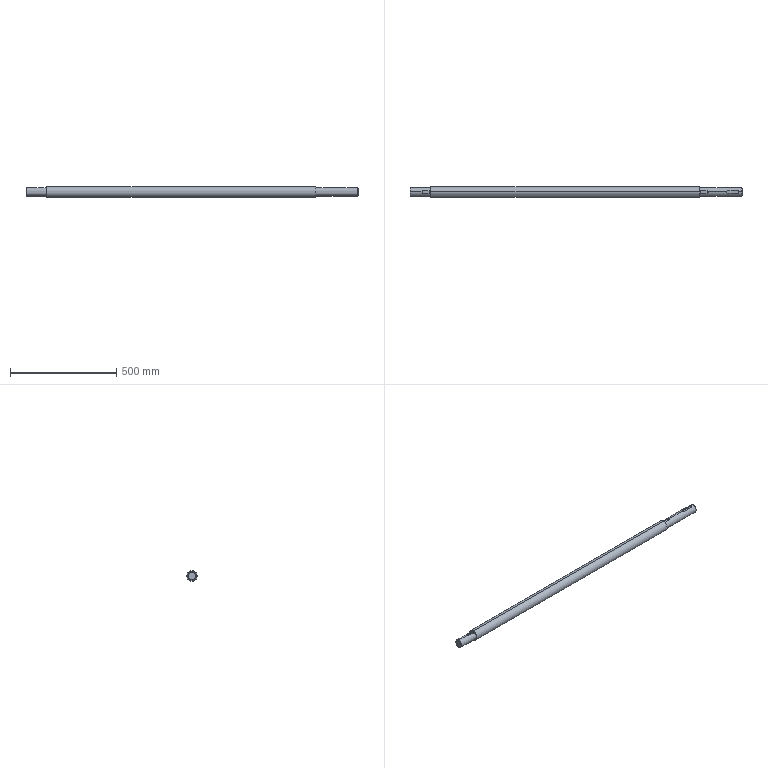Part | STEP file | Produce dryer mesh belt driving shaft | 1 solid | 32 faces | box 1562 x 50 x 50 mm | volume 2850228 mm3 | cylinder 15 | plane 13 | cone 4 | commonest cylinder face diameters 12 x9 40 x4 50 x2
STEP:
#1=CARTESIAN_POINT('',(832.25,0.,-18.));
#2=VERTEX_POINT('',#1);
#3=CARTESIAN_POINT('',(832.25,0.,18.));
#4=VERTEX_POINT('',#3);
#5=CARTESIAN_POINT('',(832.25,0.,0.));
#6=DIRECTION('',(1.,0.,0.));
#7=DIRECTION('',(0.,0.,1.));
#8=AXIS2_PLACEMENT_3D('',#5,#6,#7);
#9=CIRCLE('',#8,18.);
#10=EDGE_CURVE('',#2,#4,#9,.T.);
#11=ORIENTED_EDGE('',*,*,#10,.F.);
#12=CARTESIAN_POINT('',(830.25,0.,-20.));
#13=VERTEX_POINT('',#12);
#14=CARTESIAN_POINT('',(830.25,0.,-20.));
#15=DIRECTION('',(-0.7071,0.,-0.7071));
#16=VECTOR('',#15,1000.);
#17=LINE('',#14,#16);
#18=EDGE_CURVE('',#2,#13,#17,.T.);
#19=ORIENTED_EDGE('',*,*,#18,.T.);
#20=CARTESIAN_POINT('',(830.25,0.,20.));
#21=VERTEX_POINT('',#20);
#22=CARTESIAN_POINT('',(830.25,0.,0.));
#23=DIRECTION('',(-1.,0.,0.));
#24=DIRECTION('',(0.,0.,1.));
#25=AXIS2_PLACEMENT_3D('',#22,#23,#24);
#26=CIRCLE('',#25,20.);
#27=EDGE_CURVE('',#21,#13,#26,.T.);
#28=ORIENTED_EDGE('',*,*,#27,.F.);
#29=CARTESIAN_POINT('',(830.25,0.,20.));
#30=DIRECTION('',(-0.7071,0.,0.7071));
#31=VECTOR('',#30,1000.);
#32=LINE('',#29,#31);
#33=EDGE_CURVE('',#4,#21,#32,.T.);
#34=ORIENTED_EDGE('',*,*,#33,.F.);
#35=EDGE_LOOP('',(#11,#19,#28,#34));
#36=FACE_OUTER_BOUND('',#35,.T.);
#37=CARTESIAN_POINT('',(830.25,0.,0.));
#38=DIRECTION('',(-1.,0.,0.));
#39=DIRECTION('',(0.,0.,1.));
#40=AXIS2_PLACEMENT_3D('',#37,#38,#39);
#41=CONICAL_SURFACE('',#40,20.,0.7854);
#42=ADVANCED_FACE('',(#36),#41,.T.);
#43=CARTESIAN_POINT('',(-730.25,0.,18.));
#44=VERTEX_POINT('',#43);
#45=CARTESIAN_POINT('',(-730.25,0.,-18.));
#46=VERTEX_POINT('',#45);
#47=CARTESIAN_POINT('',(-730.25,0.,0.));
#48=DIRECTION('',(-1.,0.,0.));
#49=DIRECTION('',(0.,0.,-1.));
#50=AXIS2_PLACEMENT_3D('',#47,#48,#49);
#51=CIRCLE('',#50,18.);
#52=EDGE_CURVE('',#44,#46,#51,.T.);
#53=ORIENTED_EDGE('',*,*,#52,.F.);
#54=CARTESIAN_POINT('',(-728.25,0.,20.));
#55=VERTEX_POINT('',#54);
#56=CARTESIAN_POINT('',(-730.25,0.,18.));
#57=DIRECTION('',(0.7071,0.,0.7071));
#58=VECTOR('',#57,1000.);
#59=LINE('',#56,#58);
#60=EDGE_CURVE('',#44,#55,#59,.T.);
#61=ORIENTED_EDGE('',*,*,#60,.T.);
#62=CARTESIAN_POINT('',(-728.25,0.,-20.));
#63=VERTEX_POINT('',#62);
#64=CARTESIAN_POINT('',(-728.25,0.,0.));
#65=DIRECTION('',(1.,0.,0.));
#66=DIRECTION('',(0.,0.,-1.));
#67=AXIS2_PLACEMENT_3D('',#64,#65,#66);
#68=CIRCLE('',#67,20.);
#69=EDGE_CURVE('',#63,#55,#68,.T.);
#70=ORIENTED_EDGE('',*,*,#69,.F.);
#71=CARTESIAN_POINT('',(-730.25,0.,-18.));
#72=DIRECTION('',(0.7071,0.,-0.7071));
#73=VECTOR('',#72,1000.);
#74=LINE('',#71,#73);
#75=EDGE_CURVE('',#46,#63,#74,.T.);
#76=ORIENTED_EDGE('',*,*,#75,.F.);
#77=EDGE_LOOP('',(#53,#61,#70,#76));
#78=FACE_OUTER_BOUND('',#77,.T.);
#79=CARTESIAN_POINT('',(-730.25,0.,0.));
#80=DIRECTION('',(1.,0.,0.));
#81=DIRECTION('',(0.,0.,-1.));
#82=AXIS2_PLACEMENT_3D('',#79,#80,#81);
#83=CONICAL_SURFACE('',#82,18.,0.7854);
#84=ADVANCED_FACE('',(#78),#83,.T.);
#85=CARTESIAN_POINT('',(673.75,0.,15.));
#86=VERTEX_POINT('',#85);
#87=CARTESIAN_POINT('',(667.75,6.,15.));
#88=VERTEX_POINT('',#87);
#89=CARTESIAN_POINT('',(667.75,0.,15.));
#90=DIRECTION('',(0.,0.,1.));
#91=DIRECTION('',(-1.,0.,0.));
#92=AXIS2_PLACEMENT_3D('',#89,#90,#91);
#93=CIRCLE('',#92,6.);
#94=EDGE_CURVE('',#86,#88,#93,.T.);
#95=ORIENTED_EDGE('',*,*,#94,.F.);
#96=CARTESIAN_POINT('',(673.75,0.,20.));
#97=VERTEX_POINT('',#96);
#98=CARTESIAN_POINT('',(673.75,0.,15.));
#99=DIRECTION('',(0.,0.,1.));
#100=VECTOR('',#99,1000.);
#101=LINE('',#98,#100);
#102=EDGE_CURVE('',#86,#97,#101,.T.);
#103=ORIENTED_EDGE('',*,*,#102,.T.);
#104=CARTESIAN_POINT('',(667.75,6.,19.079));
#105=VERTEX_POINT('',#104);
#106=CARTESIAN_POINT('',(667.75,6.,19.079));
#107=CARTESIAN_POINT('',(668.145,6.,19.079));
#108=CARTESIAN_POINT('',(668.536,5.961,19.091));
#109=CARTESIAN_POINT('',(669.116,5.846,19.127));
#110=CARTESIAN_POINT('',(669.309,5.797,19.141));
#111=CARTESIAN_POINT('',(669.688,5.682,19.176));
#112=CARTESIAN_POINT('',(669.873,5.615,19.196));
#113=CARTESIAN_POINT('',(670.415,5.39,19.261));
#114=CARTESIAN_POINT('',(670.759,5.206,19.312));
#115=CARTESIAN_POINT('',(671.415,4.767,19.425));
#116=CARTESIAN_POINT('',(671.716,4.519,19.485));
#117=CARTESIAN_POINT('',(672.129,4.107,19.574));
#118=CARTESIAN_POINT('',(672.26,3.962,19.604));
#119=CARTESIAN_POINT('',(672.509,3.66,19.663));
#120=CARTESIAN_POINT('',(672.627,3.501,19.692));
#121=CARTESIAN_POINT('',(672.953,3.013,19.775));
#122=CARTESIAN_POINT('',(673.138,2.67,19.824));
#123=CARTESIAN_POINT('',(673.439,1.946,19.908));
#124=CARTESIAN_POINT('',(673.556,1.563,19.943));
#125=CARTESIAN_POINT('',(673.711,0.7911,19.988));
#126=CARTESIAN_POINT('',(673.75,0.3988,20.));
#127=CARTESIAN_POINT('',(673.75,0.,20.));
#128=B_SPLINE_CURVE_WITH_KNOTS('',3,(#106,#107,#108,#109,#110,#111,#112,#113,#114,#115,#116,#117,#118,#119,#120,#121,#122,#123,#124,#125,#126,#127),.UNSPECIFIED.,.F.,.F.,(4,2,2,2,2,2,2,2,2,2,4),(0.0283,0.02948,0.03007,0.03066,0.03184,0.03302,0.0336,0.03419,0.03537,0.03655,0.03773),.UNSPECIFIED.);
#129=EDGE_CURVE('',#105,#97,#128,.T.);
#130=ORIENTED_EDGE('',*,*,#129,.F.);
#131=CARTESIAN_POINT('',(667.75,6.,15.));
#132=DIRECTION('',(0.,0.,1.));
#133=VECTOR('',#132,1000.);
#134=LINE('',#131,#133);
#135=EDGE_CURVE('',#88,#105,#134,.T.);
#136=ORIENTED_EDGE('',*,*,#135,.F.);
#137=EDGE_LOOP('',(#95,#103,#130,#136));
#138=FACE_OUTER_BOUND('',#137,.T.);
#139=CARTESIAN_POINT('',(667.75,0.,15.));
#140=DIRECTION('',(0.,0.,1.));
#141=DIRECTION('',(1.,0.,0.));
#142=AXIS2_PLACEMENT_3D('',#139,#140,#141);
#143=CYLINDRICAL_SURFACE('',#142,6.);
#144=ADVANCED_FACE('',(#138),#143,.F.);
#145=CARTESIAN_POINT('',(818.25,0.,15.));
#146=VERTEX_POINT('',#145);
#147=CARTESIAN_POINT('',(812.25,6.,15.));
#148=VERTEX_POINT('',#147);
#149=CARTESIAN_POINT('',(812.25,0.,15.));
#150=DIRECTION('',(0.,0.,1.));
#151=DIRECTION('',(1.,0.,0.));
#152=AXIS2_PLACEMENT_3D('',#149,#150,#151);
#153=CIRCLE('',#152,6.);
#154=EDGE_CURVE('',#146,#148,#153,.T.);
#155=ORIENTED_EDGE('',*,*,#154,.F.);
#156=CARTESIAN_POINT('',(818.25,0.,20.));
#157=VERTEX_POINT('',#156);
#158=CARTESIAN_POINT('',(818.25,0.,15.));
#159=DIRECTION('',(0.,0.,1.));
#160=VECTOR('',#159,1000.);
#161=LINE('',#158,#160);
#162=EDGE_CURVE('',#146,#157,#161,.T.);
#163=ORIENTED_EDGE('',*,*,#162,.T.);
#164=CARTESIAN_POINT('',(812.25,6.,19.079));
#165=VERTEX_POINT('',#164);
#166=CARTESIAN_POINT('',(812.25,6.,19.079));
#167=CARTESIAN_POINT('',(812.645,6.,19.079));
#168=CARTESIAN_POINT('',(813.036,5.961,19.091));
#169=CARTESIAN_POINT('',(813.616,5.846,19.127));
#170=CARTESIAN_POINT('',(813.809,5.797,19.141));
#171=CARTESIAN_POINT('',(814.188,5.682,19.176));
#172=CARTESIAN_POINT('',(814.373,5.615,19.196));
#173=CARTESIAN_POINT('',(814.915,5.39,19.261));
#174=CARTESIAN_POINT('',(815.259,5.206,19.312));
#175=CARTESIAN_POINT('',(815.915,4.767,19.425));
#176=CARTESIAN_POINT('',(816.216,4.519,19.485));
#177=CARTESIAN_POINT('',(816.629,4.107,19.574));
#178=CARTESIAN_POINT('',(816.76,3.962,19.604));
#179=CARTESIAN_POINT('',(817.009,3.66,19.663));
#180=CARTESIAN_POINT('',(817.127,3.501,19.692));
#181=CARTESIAN_POINT('',(817.453,3.013,19.775));
#182=CARTESIAN_POINT('',(817.638,2.67,19.824));
#183=CARTESIAN_POINT('',(817.939,1.946,19.908));
#184=CARTESIAN_POINT('',(818.056,1.563,19.943));
#185=CARTESIAN_POINT('',(818.211,0.7911,19.988));
#186=CARTESIAN_POINT('',(818.25,0.3988,20.));
#187=CARTESIAN_POINT('',(818.25,0.,20.));
#188=B_SPLINE_CURVE_WITH_KNOTS('',3,(#166,#167,#168,#169,#170,#171,#172,#173,#174,#175,#176,#177,#178,#179,#180,#181,#182,#183,#184,#185,#186,#187),.UNSPECIFIED.,.F.,.F.,(4,2,2,2,2,2,2,2,2,2,4),(0.0283,0.02948,0.03007,0.03066,0.03184,0.03302,0.0336,0.03419,0.03537,0.03655,0.03773),.UNSPECIFIED.);
#189=EDGE_CURVE('',#165,#157,#188,.T.);
#190=ORIENTED_EDGE('',*,*,#189,.F.);
#191=CARTESIAN_POINT('',(812.25,6.,15.));
#192=DIRECTION('',(0.,0.,1.));
#193=VECTOR('',#192,1000.);
#194=LINE('',#191,#193);
#195=EDGE_CURVE('',#148,#165,#194,.T.);
#196=ORIENTED_EDGE('',*,*,#195,.F.);
#197=EDGE_LOOP('',(#155,#163,#190,#196));
#198=FACE_OUTER_BOUND('',#197,.T.);
#199=CARTESIAN_POINT('',(812.25,0.,15.));
#200=DIRECTION('',(0.,0.,1.));
#201=DIRECTION('',(1.,0.,0.));
#202=AXIS2_PLACEMENT_3D('',#199,#200,#201);
#203=CYLINDRICAL_SURFACE('',#202,6.);
#204=ADVANCED_FACE('',(#198),#203,.F.);
#205=CARTESIAN_POINT('',(-634.75,0.,15.));
#206=VERTEX_POINT('',#205);
#207=CARTESIAN_POINT('',(-640.75,6.,15.));
#208=VERTEX_POINT('',#207);
#209=CARTESIAN_POINT('',(-640.75,0.,15.));
#210=DIRECTION('',(0.,0.,1.));
#211=DIRECTION('',(1.,0.,0.));
#212=AXIS2_PLACEMENT_3D('',#209,#210,#211);
#213=CIRCLE('',#212,6.);
#214=EDGE_CURVE('',#206,#208,#213,.T.);
#215=ORIENTED_EDGE('',*,*,#214,.F.);
#216=CARTESIAN_POINT('',(-634.75,0.,20.));
#217=VERTEX_POINT('',#216);
#218=CARTESIAN_POINT('',(-634.75,0.,15.));
#219=DIRECTION('',(0.,0.,1.));
#220=VECTOR('',#219,1000.);
#221=LINE('',#218,#220);
#222=EDGE_CURVE('',#206,#217,#221,.T.);
#223=ORIENTED_EDGE('',*,*,#222,.T.);
#224=CARTESIAN_POINT('',(-640.75,6.,19.079));
#225=VERTEX_POINT('',#224);
#226=CARTESIAN_POINT('',(-640.75,6.,19.079));
#227=CARTESIAN_POINT('',(-640.355,6.,19.079));
#228=CARTESIAN_POINT('',(-639.964,5.961,19.091));
#229=CARTESIAN_POINT('',(-639.384,5.846,19.127));
#230=CARTESIAN_POINT('',(-639.191,5.797,19.141));
#231=CARTESIAN_POINT('',(-638.812,5.682,19.176));
#232=CARTESIAN_POINT('',(-638.627,5.615,19.196));
#233=CARTESIAN_POINT('',(-638.085,5.39,19.261));
#234=CARTESIAN_POINT('',(-637.741,5.206,19.312));
#235=CARTESIAN_POINT('',(-637.085,4.767,19.425));
#236=CARTESIAN_POINT('',(-636.784,4.519,19.485));
#237=CARTESIAN_POINT('',(-636.371,4.107,19.574));
#238=CARTESIAN_POINT('',(-636.24,3.962,19.604));
#239=CARTESIAN_POINT('',(-635.991,3.66,19.663));
#240=CARTESIAN_POINT('',(-635.873,3.501,19.692));
#241=CARTESIAN_POINT('',(-635.547,3.013,19.775));
#242=CARTESIAN_POINT('',(-635.362,2.67,19.824));
#243=CARTESIAN_POINT('',(-635.061,1.946,19.908));
#244=CARTESIAN_POINT('',(-634.944,1.563,19.943));
#245=CARTESIAN_POINT('',(-634.789,0.7911,19.988));
#246=CARTESIAN_POINT('',(-634.75,0.3988,20.));
#247=CARTESIAN_POINT('',(-634.75,0.,20.));
#248=B_SPLINE_CURVE_WITH_KNOTS('',3,(#226,#227,#228,#229,#230,#231,#232,#233,#234,#235,#236,#237,#238,#239,#240,#241,#242,#243,#244,#245,#246,#247),.UNSPECIFIED.,.F.,.F.,(4,2,2,2,2,2,2,2,2,2,4),(0.0283,0.02948,0.03007,0.03066,0.03184,0.03302,0.0336,0.03419,0.03537,0.03655,0.03773),.UNSPECIFIED.);
#249=EDGE_CURVE('',#225,#217,#248,.T.);
#250=ORIENTED_EDGE('',*,*,#249,.F.);
#251=CARTESIAN_POINT('',(-640.75,6.,15.));
#252=DIRECTION('',(0.,0.,1.));
#253=VECTOR('',#252,1000.);
#254=LINE('',#251,#253);
#255=EDGE_CURVE('',#208,#225,#254,.T.);
#256=ORIENTED_EDGE('',*,*,#255,.F.);
#257=EDGE_LOOP('',(#215,#223,#250,#256));
#258=FACE_OUTER_BOUND('',#257,.T.);
#259=CARTESIAN_POINT('',(-640.75,0.,15.));
#260=DIRECTION('',(0.,0.,1.));
#261=DIRECTION('',(1.,0.,0.));
#262=AXIS2_PLACEMENT_3D('',#259,#260,#261);
#263=CYLINDRICAL_SURFACE('',#262,6.);
#264=ADVANCED_FACE('',(#258),#263,.F.);
#265=CARTESIAN_POINT('',(-632.75,0.,20.));
#266=VERTEX_POINT('',#265);
#267=CARTESIAN_POINT('',(-632.75,0.,-20.));
#268=VERTEX_POINT('',#267);
#269=CARTESIAN_POINT('',(-632.75,0.,0.));
#270=DIRECTION('',(-1.,0.,0.));
#271=DIRECTION('',(0.,0.,1.));
#272=AXIS2_PLACEMENT_3D('',#269,#270,#271);
#273=CIRCLE('',#272,20.);
#274=EDGE_CURVE('',#266,#268,#273,.T.);
#275=ORIENTED_EDGE('',*,*,#274,.T.);
#276=CARTESIAN_POINT('',(-832.25,0.,-20.));
#277=DIRECTION('',(-1.,0.,0.));
#278=VECTOR('',#277,1000.);
#279=LINE('',#276,#278);
#280=EDGE_CURVE('',#268,#63,#279,.T.);
#281=ORIENTED_EDGE('',*,*,#280,.T.);
#282=ORIENTED_EDGE('',*,*,#69,.T.);
#283=CARTESIAN_POINT('',(-673.75,0.,20.));
#284=VERTEX_POINT('',#283);
#285=CARTESIAN_POINT('',(-832.25,0.,20.));
#286=DIRECTION('',(-1.,0.,0.));
#287=VECTOR('',#286,1000.);
#288=LINE('',#285,#287);
#289=EDGE_CURVE('',#284,#55,#288,.T.);
#290=ORIENTED_EDGE('',*,*,#289,.F.);
#291=CARTESIAN_POINT('',(-667.75,6.,19.079));
#292=VERTEX_POINT('',#291);
#293=CARTESIAN_POINT('',(-673.75,0.,20.));
#294=CARTESIAN_POINT('',(-673.75,0.3936,20.));
#295=CARTESIAN_POINT('',(-673.71,0.7934,19.988));
#296=CARTESIAN_POINT('',(-673.556,1.564,19.942));
#297=CARTESIAN_POINT('',(-673.442,1.939,19.909));
#298=CARTESIAN_POINT('',(-673.139,2.668,19.825));
#299=CARTESIAN_POINT('',(-672.952,3.015,19.774));
#300=CARTESIAN_POINT('',(-672.627,3.5,19.692));
#301=CARTESIAN_POINT('',(-672.511,3.657,19.664));
#302=CARTESIAN_POINT('',(-672.263,3.959,19.605));
#303=CARTESIAN_POINT('',(-672.13,4.105,19.575));
#304=CARTESIAN_POINT('',(-671.715,4.52,19.485));
#305=CARTESIAN_POINT('',(-671.415,4.766,19.425));
#306=CARTESIAN_POINT('',(-670.768,5.201,19.313));
#307=CARTESIAN_POINT('',(-670.417,5.389,19.261));
#308=CARTESIAN_POINT('',(-669.695,5.69,19.174));
#309=CARTESIAN_POINT('',(-669.321,5.804,19.139));
#310=CARTESIAN_POINT('',(-668.547,5.96,19.092));
#311=CARTESIAN_POINT('',(-668.149,6.,19.079));
#312=CARTESIAN_POINT('',(-667.75,6.,19.079));
#313=B_SPLINE_CURVE_WITH_KNOTS('',3,(#293,#294,#295,#296,#297,#298,#299,#300,#301,#302,#303,#304,#305,#306,#307,#308,#309,#310,#311,#312),.UNSPECIFIED.,.F.,.F.,(4,2,2,2,2,2,2,2,2,4),(0.009436,0.01061,0.01179,0.01297,0.01356,0.01415,0.01533,0.0165,0.01768,0.01886),.UNSPECIFIED.);
#314=EDGE_CURVE('',#284,#292,#313,.T.);
#315=ORIENTED_EDGE('',*,*,#314,.T.);
#316=CARTESIAN_POINT('',(-832.25,6.,19.079));
#317=DIRECTION('',(1.,0.,0.));
#318=VECTOR('',#317,1000.);
#319=LINE('',#316,#318);
#320=EDGE_CURVE('',#292,#225,#319,.T.);
#321=ORIENTED_EDGE('',*,*,#320,.T.);
#322=ORIENTED_EDGE('',*,*,#249,.T.);
#323=CARTESIAN_POINT('',(-832.25,0.,20.));
#324=DIRECTION('',(-1.,0.,0.));
#325=VECTOR('',#324,1000.);
#326=LINE('',#323,#325);
#327=EDGE_CURVE('',#266,#217,#326,.T.);
#328=ORIENTED_EDGE('',*,*,#327,.F.);
#329=EDGE_LOOP('',(#275,#281,#282,#290,#315,#321,#322,#328));
#330=FACE_OUTER_BOUND('',#329,.T.);
#331=CARTESIAN_POINT('',(-832.25,0.,0.));
#332=DIRECTION('',(-1.,0.,0.));
#333=DIRECTION('',(0.,0.,1.));
#334=AXIS2_PLACEMENT_3D('',#331,#332,#333);
#335=CYLINDRICAL_SURFACE('',#334,20.);
#336=ADVANCED_FACE('',(#330),#335,.T.);
#337=CARTESIAN_POINT('',(632.75,0.,25.));
#338=VERTEX_POINT('',#337);
#339=CARTESIAN_POINT('',(632.75,0.,-25.));
#340=VERTEX_POINT('',#339);
#341=CARTESIAN_POINT('',(632.75,0.,0.));
#342=DIRECTION('',(-1.,0.,0.));
#343=DIRECTION('',(0.,0.,1.));
#344=AXIS2_PLACEMENT_3D('',#341,#342,#343);
#345=CIRCLE('',#344,25.);
#346=EDGE_CURVE('',#338,#340,#345,.T.);
#347=ORIENTED_EDGE('',*,*,#346,.T.);
#348=CARTESIAN_POINT('',(-632.75,0.,-25.));
#349=VERTEX_POINT('',#348);
#350=CARTESIAN_POINT('',(-832.25,0.,-25.));
#351=DIRECTION('',(-1.,0.,0.));
#352=VECTOR('',#351,1000.);
#353=LINE('',#350,#352);
#354=EDGE_CURVE('',#340,#349,#353,.T.);
#355=ORIENTED_EDGE('',*,*,#354,.T.);
#356=CARTESIAN_POINT('',(-632.75,0.,25.));
#357=VERTEX_POINT('',#356);
#358=CARTESIAN_POINT('',(-632.75,0.,0.));
#359=DIRECTION('',(-1.,0.,0.));
#360=DIRECTION('',(0.,0.,1.));
#361=AXIS2_PLACEMENT_3D('',#358,#359,#360);
#362=CIRCLE('',#361,25.);
#363=EDGE_CURVE('',#357,#349,#362,.T.);
#364=ORIENTED_EDGE('',*,*,#363,.F.);
#365=CARTESIAN_POINT('',(-832.25,0.,25.));
#366=DIRECTION('',(-1.,0.,0.));
#367=VECTOR('',#366,1000.);
#368=LINE('',#365,#367);
#369=EDGE_CURVE('',#338,#357,#368,.T.);
#370=ORIENTED_EDGE('',*,*,#369,.F.);
#371=EDGE_LOOP('',(#347,#355,#364,#370));
#372=FACE_OUTER_BOUND('',#371,.T.);
#373=CARTESIAN_POINT('',(-832.25,0.,0.));
#374=DIRECTION('',(-1.,0.,0.));
#375=DIRECTION('',(0.,0.,1.));
#376=AXIS2_PLACEMENT_3D('',#373,#374,#375);
#377=CYLINDRICAL_SURFACE('',#376,25.);
#378=ADVANCED_FACE('',(#372),#377,.T.);
#379=ORIENTED_EDGE('',*,*,#27,.T.);
#380=CARTESIAN_POINT('',(632.75,0.,-20.));
#381=VERTEX_POINT('',#380);
#382=CARTESIAN_POINT('',(-832.25,0.,-20.));
#383=DIRECTION('',(-1.,0.,0.));
#384=VECTOR('',#383,1000.);
#385=LINE('',#382,#384);
#386=EDGE_CURVE('',#13,#381,#385,.T.);
#387=ORIENTED_EDGE('',*,*,#386,.T.);
#388=CARTESIAN_POINT('',(632.75,0.,20.));
#389=VERTEX_POINT('',#388);
#390=CARTESIAN_POINT('',(632.75,0.,0.));
#391=DIRECTION('',(-1.,0.,0.));
#392=DIRECTION('',(0.,0.,1.));
#393=AXIS2_PLACEMENT_3D('',#390,#391,#392);
#394=CIRCLE('',#393,20.);
#395=EDGE_CURVE('',#389,#381,#394,.T.);
#396=ORIENTED_EDGE('',*,*,#395,.F.);
#397=CARTESIAN_POINT('',(634.75,0.,20.));
#398=VERTEX_POINT('',#397);
#399=CARTESIAN_POINT('',(-832.25,0.,20.));
#400=DIRECTION('',(-1.,0.,0.));
#401=VECTOR('',#400,1000.);
#402=LINE('',#399,#401);
#403=EDGE_CURVE('',#398,#389,#402,.T.);
#404=ORIENTED_EDGE('',*,*,#403,.F.);
#405=CARTESIAN_POINT('',(640.75,6.,19.079));
#406=VERTEX_POINT('',#405);
#407=CARTESIAN_POINT('',(634.75,0.,20.));
#408=CARTESIAN_POINT('',(634.75,0.3936,20.));
#409=CARTESIAN_POINT('',(634.79,0.7934,19.988));
#410=CARTESIAN_POINT('',(634.944,1.564,19.942));
#411=CARTESIAN_POINT('',(635.058,1.939,19.909));
#412=CARTESIAN_POINT('',(635.361,2.668,19.825));
#413=CARTESIAN_POINT('',(635.548,3.015,19.774));
#414=CARTESIAN_POINT('',(635.873,3.5,19.692));
#415=CARTESIAN_POINT('',(635.989,3.657,19.664));
#416=CARTESIAN_POINT('',(636.237,3.959,19.605));
#417=CARTESIAN_POINT('',(636.37,4.105,19.575));
#418=CARTESIAN_POINT('',(636.785,4.52,19.485));
#419=CARTESIAN_POINT('',(637.085,4.766,19.425));
#420=CARTESIAN_POINT('',(637.732,5.201,19.313));
#421=CARTESIAN_POINT('',(638.083,5.389,19.261));
#422=CARTESIAN_POINT('',(638.805,5.69,19.174));
#423=CARTESIAN_POINT('',(639.179,5.804,19.139));
#424=CARTESIAN_POINT('',(639.953,5.96,19.092));
#425=CARTESIAN_POINT('',(640.351,6.,19.079));
#426=CARTESIAN_POINT('',(640.75,6.,19.079));
#427=B_SPLINE_CURVE_WITH_KNOTS('',3,(#407,#408,#409,#410,#411,#412,#413,#414,#415,#416,#417,#418,#419,#420,#421,#422,#423,#424,#425,#426),.UNSPECIFIED.,.F.,.F.,(4,2,2,2,2,2,2,2,2,4),(0.009436,0.01061,0.01179,0.01297,0.01356,0.01415,0.01533,0.0165,0.01768,0.01886),.UNSPECIFIED.);
#428=EDGE_CURVE('',#398,#406,#427,.T.);
#429=ORIENTED_EDGE('',*,*,#428,.T.);
#430=CARTESIAN_POINT('',(-832.25,6.,19.079));
#431=DIRECTION('',(1.,0.,0.));
#432=VECTOR('',#431,1000.);
#433=LINE('',#430,#432);
#434=EDGE_CURVE('',#406,#105,#433,.T.);
#435=ORIENTED_EDGE('',*,*,#434,.T.);
#436=ORIENTED_EDGE('',*,*,#129,.T.);
#437=CARTESIAN_POINT('',(759.25,0.,20.));
#438=VERTEX_POINT('',#437);
#439=CARTESIAN_POINT('',(-832.25,0.,20.));
#440=DIRECTION('',(-1.,0.,0.));
#441=VECTOR('',#440,1000.);
#442=LINE('',#439,#441);
#443=EDGE_CURVE('',#438,#97,#442,.T.);
#444=ORIENTED_EDGE('',*,*,#443,.F.);
#445=CARTESIAN_POINT('',(765.25,6.,19.079));
#446=VERTEX_POINT('',#445);
#447=CARTESIAN_POINT('',(759.25,0.,20.));
#448=CARTESIAN_POINT('',(759.25,0.393,20.));
#449=CARTESIAN_POINT('',(759.289,0.7872,19.988));
#450=CARTESIAN_POINT('',(759.444,1.566,19.942));
#451=CARTESIAN_POINT('',(759.559,1.941,19.909));
#452=CARTESIAN_POINT('',(759.86,2.665,19.825));
#453=CARTESIAN_POINT('',(760.048,3.016,19.774));
#454=CARTESIAN_POINT('',(760.483,3.665,19.664));
#455=CARTESIAN_POINT('',(760.73,3.965,19.605));
#456=CARTESIAN_POINT('',(761.145,4.381,19.515));
#457=CARTESIAN_POINT('',(761.292,4.514,19.484));
#458=CARTESIAN_POINT('',(761.594,4.762,19.425));
#459=CARTESIAN_POINT('',(761.751,4.878,19.396));
#460=CARTESIAN_POINT('',(762.236,5.203,19.313));
#461=CARTESIAN_POINT('',(762.58,5.388,19.261));
#462=CARTESIAN_POINT('',(763.312,5.692,19.174));
#463=CARTESIAN_POINT('',(763.687,5.806,19.139));
#464=CARTESIAN_POINT('',(764.264,5.922,19.103));
#465=CARTESIAN_POINT('',(764.458,5.951,19.094));
#466=CARTESIAN_POINT('',(764.852,5.99,19.082));
#467=CARTESIAN_POINT('',(765.052,6.,19.079));
#468=CARTESIAN_POINT('',(765.25,6.,19.079));
#469=B_SPLINE_CURVE_WITH_KNOTS('',3,(#447,#448,#449,#450,#451,#452,#453,#454,#455,#456,#457,#458,#459,#460,#461,#462,#463,#464,#465,#466,#467,#468),.UNSPECIFIED.,.F.,.F.,(4,2,2,2,2,2,2,2,2,2,4),(0.01887,0.02005,0.02123,0.0224,0.02358,0.02417,0.02476,0.02594,0.02712,0.02771,0.0283),.UNSPECIFIED.);
#470=EDGE_CURVE('',#438,#446,#469,.T.);
#471=ORIENTED_EDGE('',*,*,#470,.T.);
#472=CARTESIAN_POINT('',(-832.25,6.,19.079));
#473=DIRECTION('',(1.,0.,0.));
#474=VECTOR('',#473,1000.);
#475=LINE('',#472,#474);
#476=EDGE_CURVE('',#446,#165,#475,.T.);
#477=ORIENTED_EDGE('',*,*,#476,.T.);
#478=ORIENTED_EDGE('',*,*,#189,.T.);
#479=CARTESIAN_POINT('',(-832.25,0.,20.));
#480=DIRECTION('',(-1.,0.,0.));
#481=VECTOR('',#480,1000.);
#482=LINE('',#479,#481);
#483=EDGE_CURVE('',#21,#157,#482,.T.);
#484=ORIENTED_EDGE('',*,*,#483,.F.);
#485=EDGE_LOOP('',(#379,#387,#396,#404,#429,#435,#436,#444,#471,#477,#478,#484));
#486=FACE_OUTER_BOUND('',#485,.T.);
#487=CARTESIAN_POINT('',(-832.25,0.,0.));
#488=DIRECTION('',(-1.,0.,0.));
#489=DIRECTION('',(0.,0.,1.));
#490=AXIS2_PLACEMENT_3D('',#487,#488,#489);
#491=CYLINDRICAL_SURFACE('',#490,20.);
#492=ADVANCED_FACE('',(#486),#491,.T.);
#493=CARTESIAN_POINT('',(832.25,0.,0.));
#494=DIRECTION('',(1.,0.,0.));
#495=DIRECTION('',(0.,0.,1.));
#496=AXIS2_PLACEMENT_3D('',#493,#494,#495);
#497=CIRCLE('',#496,18.);
#498=EDGE_CURVE('',#4,#2,#497,.T.);
#499=ORIENTED_EDGE('',*,*,#498,.T.);
#500=ORIENTED_EDGE('',*,*,#10,.T.);
#501=EDGE_LOOP('',(#499,#500));
#502=FACE_OUTER_BOUND('',#501,.T.);
#503=CARTESIAN_POINT('',(832.25,0.,0.));
#504=DIRECTION('',(-1.,0.,0.));
#505=DIRECTION('',(0.,0.,1.));
#506=AXIS2_PLACEMENT_3D('',#503,#504,#505);
#507=PLANE('',#506);
#508=ADVANCED_FACE('',(#502),#507,.F.);
#509=ORIENTED_EDGE('',*,*,#386,.F.);
#510=CARTESIAN_POINT('',(830.25,0.,0.));
#511=DIRECTION('',(-1.,0.,0.));
#512=DIRECTION('',(0.,0.,1.));
#513=AXIS2_PLACEMENT_3D('',#510,#511,#512);
#514=CIRCLE('',#513,20.);
#515=EDGE_CURVE('',#13,#21,#514,.T.);
#516=ORIENTED_EDGE('',*,*,#515,.T.);
#517=ORIENTED_EDGE('',*,*,#483,.T.);
#518=CARTESIAN_POINT('',(812.25,-6.,19.079));
#519=VERTEX_POINT('',#518);
#520=CARTESIAN_POINT('',(818.25,0.,20.));
#521=CARTESIAN_POINT('',(818.25,-0.399,20.));
#522=CARTESIAN_POINT('',(818.211,-0.7909,19.988));
#523=CARTESIAN_POINT('',(818.095,-1.369,19.954));
#524=CARTESIAN_POINT('',(818.047,-1.56,19.94));
#525=CARTESIAN_POINT('',(817.932,-1.938,19.907));
#526=CARTESIAN_POINT('',(817.864,-2.125,19.888));
#527=CARTESIAN_POINT('',(817.638,-2.67,19.824));
#528=CARTESIAN_POINT('',(817.453,-3.013,19.774));
#529=CARTESIAN_POINT('',(817.126,-3.501,19.692));
#530=CARTESIAN_POINT('',(817.008,-3.66,19.663));
#531=CARTESIAN_POINT('',(816.759,-3.963,19.604));
#532=CARTESIAN_POINT('',(816.628,-4.108,19.574));
#533=CARTESIAN_POINT('',(816.215,-4.52,19.485));
#534=CARTESIAN_POINT('',(815.914,-4.768,19.425));
#535=CARTESIAN_POINT('',(815.259,-5.206,19.312));
#536=CARTESIAN_POINT('',(814.913,-5.391,19.26));
#537=CARTESIAN_POINT('',(814.372,-5.616,19.196));
#538=CARTESIAN_POINT('',(814.188,-5.682,19.176));
#539=CARTESIAN_POINT('',(813.811,-5.797,19.142));
#540=CARTESIAN_POINT('',(813.617,-5.846,19.127));
#541=CARTESIAN_POINT('',(813.035,-5.962,19.091));
#542=CARTESIAN_POINT('',(812.644,-6.,19.079));
#543=CARTESIAN_POINT('',(812.25,-6.,19.079));
#544=B_SPLINE_CURVE_WITH_KNOTS('',3,(#520,#521,#522,#523,#524,#525,#526,#527,#528,#529,#530,#531,#532,#533,#534,#535,#536,#537,#538,#539,#540,#541,#542,#543),.UNSPECIFIED.,.F.,.F.,(4,2,2,2,2,2,2,2,2,2,2,4),(0.,0.00118,0.001769,0.002359,0.003539,0.004129,0.004718,0.005898,0.007078,0.007667,0.008257,0.009437),.UNSPECIFIED.);
#545=EDGE_CURVE('',#157,#519,#544,.T.);
#546=ORIENTED_EDGE('',*,*,#545,.T.);
#547=CARTESIAN_POINT('',(765.25,-6.,19.079));
#548=VERTEX_POINT('',#547);
#549=CARTESIAN_POINT('',(-832.25,-6.,19.079));
#550=DIRECTION('',(-1.,0.,0.));
#551=VECTOR('',#550,1000.);
#552=LINE('',#549,#551);
#553=EDGE_CURVE('',#519,#548,#552,.T.);
#554=ORIENTED_EDGE('',*,*,#553,.T.);
#555=CARTESIAN_POINT('',(765.25,-6.,19.079));
#556=CARTESIAN_POINT('',(764.856,-6.,19.079));
#557=CARTESIAN_POINT('',(764.456,-5.96,19.091));
#558=CARTESIAN_POINT('',(763.685,-5.806,19.139));
#559=CARTESIAN_POINT('',(763.31,-5.691,19.174));
#560=CARTESIAN_POINT('',(762.581,-5.388,19.261));
#561=CARTESIAN_POINT('',(762.234,-5.201,19.313));
#562=CARTESIAN_POINT('',(761.749,-4.876,19.397));
#563=CARTESIAN_POINT('',(761.592,-4.76,19.426));
#564=CARTESIAN_POINT('',(761.29,-4.512,19.485));
#565=CARTESIAN_POINT('',(761.143,-4.379,19.515));
#566=CARTESIAN_POINT('',(760.728,-3.963,19.605));
#567=CARTESIAN_POINT('',(760.482,-3.663,19.664));
#568=CARTESIAN_POINT('',(760.048,-3.015,19.774));
#569=CARTESIAN_POINT('',(759.859,-2.663,19.825));
#570=CARTESIAN_POINT('',(759.559,-1.94,19.909));
#571=CARTESIAN_POINT('',(759.444,-1.566,19.942));
#572=CARTESIAN_POINT('',(759.328,-0.9847,19.977));
#573=CARTESIAN_POINT('',(759.299,-0.7868,19.985));
#574=CARTESIAN_POINT('',(759.26,-0.3931,19.997));
#575=CARTESIAN_POINT('',(759.25,-0.1965,20.));
#576=CARTESIAN_POINT('',(759.25,0.,20.));
#577=B_SPLINE_CURVE_WITH_KNOTS('',3,(#555,#556,#557,#558,#559,#560,#561,#562,#563,#564,#565,#566,#567,#568,#569,#570,#571,#572,#573,#574,#575,#576),.UNSPECIFIED.,.F.,.F.,(4,2,2,2,2,2,2,2,2,2,4),(0.009437,0.01062,0.01179,0.01297,0.01356,0.01415,0.01533,0.01651,0.01769,0.01828,0.01887),.UNSPECIFIED.);
#578=EDGE_CURVE('',#548,#438,#577,.T.);
#579=ORIENTED_EDGE('',*,*,#578,.T.);
#580=ORIENTED_EDGE('',*,*,#443,.T.);
#581=CARTESIAN_POINT('',(667.75,-6.,19.079));
#582=VERTEX_POINT('',#581);
#583=CARTESIAN_POINT('',(673.75,0.,20.));
#584=CARTESIAN_POINT('',(673.75,-0.399,20.));
#585=CARTESIAN_POINT('',(673.711,-0.7909,19.988));
#586=CARTESIAN_POINT('',(673.595,-1.369,19.954));
#587=CARTESIAN_POINT('',(673.547,-1.56,19.94));
#588=CARTESIAN_POINT('',(673.432,-1.938,19.907));
#589=CARTESIAN_POINT('',(673.364,-2.125,19.888));
#590=CARTESIAN_POINT('',(673.138,-2.67,19.824));
#591=CARTESIAN_POINT('',(672.953,-3.013,19.774));
#592=CARTESIAN_POINT('',(672.626,-3.501,19.692));
#593=CARTESIAN_POINT('',(672.508,-3.66,19.663));
#594=CARTESIAN_POINT('',(672.259,-3.963,19.604));
#595=CARTESIAN_POINT('',(672.128,-4.108,19.574));
#596=CARTESIAN_POINT('',(671.715,-4.52,19.485));
#597=CARTESIAN_POINT('',(671.414,-4.768,19.425));
#598=CARTESIAN_POINT('',(670.759,-5.206,19.312));
#599=CARTESIAN_POINT('',(670.413,-5.391,19.26));
#600=CARTESIAN_POINT('',(669.872,-5.616,19.196));
#601=CARTESIAN_POINT('',(669.688,-5.682,19.176));
#602=CARTESIAN_POINT('',(669.311,-5.797,19.142));
#603=CARTESIAN_POINT('',(669.117,-5.846,19.127));
#604=CARTESIAN_POINT('',(668.535,-5.962,19.091));
#605=CARTESIAN_POINT('',(668.144,-6.,19.079));
#606=CARTESIAN_POINT('',(667.75,-6.,19.079));
#607=B_SPLINE_CURVE_WITH_KNOTS('',3,(#583,#584,#585,#586,#587,#588,#589,#590,#591,#592,#593,#594,#595,#596,#597,#598,#599,#600,#601,#602,#603,#604,#605,#606),.UNSPECIFIED.,.F.,.F.,(4,2,2,2,2,2,2,2,2,2,2,4),(0.,0.00118,0.001769,0.002359,0.003539,0.004129,0.004718,0.005898,0.007078,0.007667,0.008257,0.009437),.UNSPECIFIED.);
#608=EDGE_CURVE('',#97,#582,#607,.T.);
#609=ORIENTED_EDGE('',*,*,#608,.T.);
#610=CARTESIAN_POINT('',(640.75,-6.,19.079));
#611=VERTEX_POINT('',#610);
#612=CARTESIAN_POINT('',(-832.25,-6.,19.079));
#613=DIRECTION('',(-1.,0.,0.));
#614=VECTOR('',#613,1000.);
#615=LINE('',#612,#614);
#616=EDGE_CURVE('',#582,#611,#615,.T.);
#617=ORIENTED_EDGE('',*,*,#616,.T.);
#618=CARTESIAN_POINT('',(640.75,-6.,19.079));
#619=CARTESIAN_POINT('',(640.351,-6.,19.079));
#620=CARTESIAN_POINT('',(639.959,-5.961,19.091));
#621=CARTESIAN_POINT('',(639.381,-5.845,19.127));
#622=CARTESIAN_POINT('',(639.191,-5.797,19.141));
#623=CARTESIAN_POINT('',(638.812,-5.682,19.176));
#624=CARTESIAN_POINT('',(638.625,-5.615,19.196));
#625=CARTESIAN_POINT('',(638.081,-5.388,19.261));
#626=CARTESIAN_POINT('',(637.737,-5.203,19.313));
#627=CARTESIAN_POINT('',(637.249,-4.877,19.397));
#628=CARTESIAN_POINT('',(637.09,-4.759,19.426));
#629=CARTESIAN_POINT('',(636.787,-4.51,19.485));
#630=CARTESIAN_POINT('',(636.643,-4.378,19.515));
#631=CARTESIAN_POINT('',(636.231,-3.966,19.605));
#632=CARTESIAN_POINT('',(635.983,-3.665,19.664));
#633=CARTESIAN_POINT('',(635.544,-3.009,19.775));
#634=CARTESIAN_POINT('',(635.359,-2.664,19.825));
#635=CARTESIAN_POINT('',(635.135,-2.122,19.888));
#636=CARTESIAN_POINT('',(635.068,-1.938,19.907));
#637=CARTESIAN_POINT('',(634.953,-1.561,19.94));
#638=CARTESIAN_POINT('',(634.904,-1.367,19.954));
#639=CARTESIAN_POINT('',(634.788,-0.7852,19.988));
#640=CARTESIAN_POINT('',(634.75,-0.3941,20.));
#641=CARTESIAN_POINT('',(634.75,0.,20.));
#642=B_SPLINE_CURVE_WITH_KNOTS('',3,(#618,#619,#620,#621,#622,#623,#624,#625,#626,#627,#628,#629,#630,#631,#632,#633,#634,#635,#636,#637,#638,#639,#640,#641),.UNSPECIFIED.,.F.,.F.,(4,2,2,2,2,2,2,2,2,2,2,4),(0.,0.00118,0.001769,0.002359,0.003539,0.004128,0.004718,0.005898,0.007077,0.007667,0.008257,0.009436),.UNSPECIFIED.);
#643=EDGE_CURVE('',#611,#398,#642,.T.);
#644=ORIENTED_EDGE('',*,*,#643,.T.);
#645=ORIENTED_EDGE('',*,*,#403,.T.);
#646=CARTESIAN_POINT('',(632.75,0.,0.));
#647=DIRECTION('',(-1.,0.,0.));
#648=DIRECTION('',(0.,0.,1.));
#649=AXIS2_PLACEMENT_3D('',#646,#647,#648);
#650=CIRCLE('',#649,20.);
#651=EDGE_CURVE('',#381,#389,#650,.T.);
#652=ORIENTED_EDGE('',*,*,#651,.F.);
#653=EDGE_LOOP('',(#509,#516,#517,#546,#554,#579,#580,#609,#617,#644,#645,#652));
#654=FACE_OUTER_BOUND('',#653,.T.);
#655=CARTESIAN_POINT('',(-832.25,0.,0.));
#656=DIRECTION('',(-1.,0.,0.));
#657=DIRECTION('',(0.,0.,1.));
#658=AXIS2_PLACEMENT_3D('',#655,#656,#657);
#659=CYLINDRICAL_SURFACE('',#658,20.);
#660=ADVANCED_FACE('',(#654),#659,.T.);
#661=ORIENTED_EDGE('',*,*,#346,.F.);
#662=CARTESIAN_POINT('',(632.75,0.,0.));
#663=DIRECTION('',(-1.,0.,0.));
#664=DIRECTION('',(0.,0.,1.));
#665=AXIS2_PLACEMENT_3D('',#662,#663,#664);
#666=CIRCLE('',#665,25.);
#667=EDGE_CURVE('',#340,#338,#666,.T.);
#668=ORIENTED_EDGE('',*,*,#667,.F.);
#669=EDGE_LOOP('',(#661,#668));
#670=FACE_OUTER_BOUND('',#669,.T.);
#671=ORIENTED_EDGE('',*,*,#395,.T.);
#672=ORIENTED_EDGE('',*,*,#651,.T.);
#673=EDGE_LOOP('',(#671,#672));
#674=FACE_BOUND('',#673,.T.);
#675=CARTESIAN_POINT('',(632.75,20.,0.));
#676=DIRECTION('',(-1.,0.,0.));
#677=DIRECTION('',(0.,0.,1.));
#678=AXIS2_PLACEMENT_3D('',#675,#676,#677);
#679=PLANE('',#678);
#680=ADVANCED_FACE('',(#670,#674),#679,.F.);
#681=ORIENTED_EDGE('',*,*,#354,.F.);
#682=ORIENTED_EDGE('',*,*,#667,.T.);
#683=ORIENTED_EDGE('',*,*,#369,.T.);
#684=CARTESIAN_POINT('',(-632.75,0.,0.));
#685=DIRECTION('',(-1.,0.,0.));
#686=DIRECTION('',(0.,0.,1.));
#687=AXIS2_PLACEMENT_3D('',#684,#685,#686);
#688=CIRCLE('',#687,25.);
#689=EDGE_CURVE('',#349,#357,#688,.T.);
#690=ORIENTED_EDGE('',*,*,#689,.F.);
#691=EDGE_LOOP('',(#681,#682,#683,#690));
#692=FACE_OUTER_BOUND('',#691,.T.);
#693=CARTESIAN_POINT('',(-832.25,0.,0.));
#694=DIRECTION('',(-1.,0.,0.));
#695=DIRECTION('',(0.,0.,1.));
#696=AXIS2_PLACEMENT_3D('',#693,#694,#695);
#697=CYLINDRICAL_SURFACE('',#696,25.);
#698=ADVANCED_FACE('',(#692),#697,.T.);
#699=ORIENTED_EDGE('',*,*,#274,.F.);
#700=CARTESIAN_POINT('',(-632.75,0.,0.));
#701=DIRECTION('',(-1.,0.,0.));
#702=DIRECTION('',(0.,0.,1.));
#703=AXIS2_PLACEMENT_3D('',#700,#701,#702);
#704=CIRCLE('',#703,20.);
#705=EDGE_CURVE('',#268,#266,#704,.T.);
#706=ORIENTED_EDGE('',*,*,#705,.F.);
#707=EDGE_LOOP('',(#699,#706));
#708=FACE_BOUND('',#707,.T.);
#709=ORIENTED_EDGE('',*,*,#363,.T.);
#710=ORIENTED_EDGE('',*,*,#689,.T.);
#711=EDGE_LOOP('',(#709,#710));
#712=FACE_OUTER_BOUND('',#711,.T.);
#713=CARTESIAN_POINT('',(-632.75,25.,0.));
#714=DIRECTION('',(1.,0.,0.));
#715=DIRECTION('',(0.,0.,-1.));
#716=AXIS2_PLACEMENT_3D('',#713,#714,#715);
#717=PLANE('',#716);
#718=ADVANCED_FACE('',(#708,#712),#717,.F.);
#719=ORIENTED_EDGE('',*,*,#280,.F.);
#720=ORIENTED_EDGE('',*,*,#705,.T.);
#721=ORIENTED_EDGE('',*,*,#327,.T.);
#722=CARTESIAN_POINT('',(-640.75,-6.,19.079));
#723=VERTEX_POINT('',#722);
#724=CARTESIAN_POINT('',(-634.75,0.,20.));
#725=CARTESIAN_POINT('',(-634.75,-0.399,20.));
#726=CARTESIAN_POINT('',(-634.789,-0.7909,19.988));
#727=CARTESIAN_POINT('',(-634.905,-1.369,19.954));
#728=CARTESIAN_POINT('',(-634.953,-1.56,19.94));
#729=CARTESIAN_POINT('',(-635.068,-1.938,19.907));
#730=CARTESIAN_POINT('',(-635.136,-2.125,19.888));
#731=CARTESIAN_POINT('',(-635.362,-2.67,19.824));
#732=CARTESIAN_POINT('',(-635.547,-3.013,19.774));
#733=CARTESIAN_POINT('',(-635.874,-3.501,19.692));
#734=CARTESIAN_POINT('',(-635.992,-3.66,19.663));
#735=CARTESIAN_POINT('',(-636.241,-3.963,19.604));
#736=CARTESIAN_POINT('',(-636.372,-4.108,19.574));
#737=CARTESIAN_POINT('',(-636.785,-4.52,19.485));
#738=CARTESIAN_POINT('',(-637.086,-4.768,19.425));
#739=CARTESIAN_POINT('',(-637.741,-5.206,19.312));
#740=CARTESIAN_POINT('',(-638.087,-5.391,19.26));
#741=CARTESIAN_POINT('',(-638.628,-5.616,19.196));
#742=CARTESIAN_POINT('',(-638.812,-5.682,19.176));
#743=CARTESIAN_POINT('',(-639.189,-5.797,19.142));
#744=CARTESIAN_POINT('',(-639.383,-5.846,19.127));
#745=CARTESIAN_POINT('',(-639.965,-5.962,19.091));
#746=CARTESIAN_POINT('',(-640.356,-6.,19.079));
#747=CARTESIAN_POINT('',(-640.75,-6.,19.079));
#748=B_SPLINE_CURVE_WITH_KNOTS('',3,(#724,#725,#726,#727,#728,#729,#730,#731,#732,#733,#734,#735,#736,#737,#738,#739,#740,#741,#742,#743,#744,#745,#746,#747),.UNSPECIFIED.,.F.,.F.,(4,2,2,2,2,2,2,2,2,2,2,4),(0.,0.00118,0.001769,0.002359,0.003539,0.004129,0.004718,0.005898,0.007078,0.007667,0.008257,0.009437),.UNSPECIFIED.);
#749=EDGE_CURVE('',#217,#723,#748,.T.);
#750=ORIENTED_EDGE('',*,*,#749,.T.);
#751=CARTESIAN_POINT('',(-667.75,-6.,19.079));
#752=VERTEX_POINT('',#751);
#753=CARTESIAN_POINT('',(-832.25,-6.,19.079));
#754=DIRECTION('',(-1.,0.,0.));
#755=VECTOR('',#754,1000.);
#756=LINE('',#753,#755);
#757=EDGE_CURVE('',#723,#752,#756,.T.);
#758=ORIENTED_EDGE('',*,*,#757,.T.);
#759=CARTESIAN_POINT('',(-667.75,-6.,19.079));
#760=CARTESIAN_POINT('',(-668.149,-6.,19.079));
#761=CARTESIAN_POINT('',(-668.541,-5.961,19.091));
#762=CARTESIAN_POINT('',(-669.119,-5.845,19.127));
#763=CARTESIAN_POINT('',(-669.309,-5.797,19.141));
#764=CARTESIAN_POINT('',(-669.688,-5.682,19.176));
#765=CARTESIAN_POINT('',(-669.875,-5.615,19.196));
#766=CARTESIAN_POINT('',(-670.419,-5.388,19.261));
#767=CARTESIAN_POINT('',(-670.763,-5.203,19.313));
#768=CARTESIAN_POINT('',(-671.251,-4.877,19.397));
#769=CARTESIAN_POINT('',(-671.41,-4.759,19.426));
#770=CARTESIAN_POINT('',(-671.713,-4.51,19.485));
#771=CARTESIAN_POINT('',(-671.857,-4.378,19.515));
#772=CARTESIAN_POINT('',(-672.269,-3.966,19.605));
#773=CARTESIAN_POINT('',(-672.517,-3.665,19.664));
#774=CARTESIAN_POINT('',(-672.956,-3.009,19.775));
#775=CARTESIAN_POINT('',(-673.141,-2.664,19.825));
#776=CARTESIAN_POINT('',(-673.365,-2.122,19.888));
#777=CARTESIAN_POINT('',(-673.432,-1.938,19.907));
#778=CARTESIAN_POINT('',(-673.547,-1.561,19.94));
#779=CARTESIAN_POINT('',(-673.596,-1.367,19.954));
#780=CARTESIAN_POINT('',(-673.712,-0.7852,19.988));
#781=CARTESIAN_POINT('',(-673.75,-0.3941,20.));
#782=CARTESIAN_POINT('',(-673.75,0.,20.));
#783=B_SPLINE_CURVE_WITH_KNOTS('',3,(#759,#760,#761,#762,#763,#764,#765,#766,#767,#768,#769,#770,#771,#772,#773,#774,#775,#776,#777,#778,#779,#780,#781,#782),.UNSPECIFIED.,.F.,.F.,(4,2,2,2,2,2,2,2,2,2,2,4),(0.,0.00118,0.001769,0.002359,0.003539,0.004128,0.004718,0.005898,0.007077,0.007667,0.008257,0.009436),.UNSPECIFIED.);
#784=EDGE_CURVE('',#752,#284,#783,.T.);
#785=ORIENTED_EDGE('',*,*,#784,.T.);
#786=ORIENTED_EDGE('',*,*,#289,.T.);
#787=CARTESIAN_POINT('',(-728.25,0.,0.));
#788=DIRECTION('',(1.,0.,0.));
#789=DIRECTION('',(0.,0.,-1.));
#790=AXIS2_PLACEMENT_3D('',#787,#788,#789);
#791=CIRCLE('',#790,20.);
#792=EDGE_CURVE('',#55,#63,#791,.T.);
#793=ORIENTED_EDGE('',*,*,#792,.T.);
#794=EDGE_LOOP('',(#719,#720,#721,#750,#758,#785,#786,#793));
#795=FACE_OUTER_BOUND('',#794,.T.);
#796=CARTESIAN_POINT('',(-832.25,0.,0.));
#797=DIRECTION('',(-1.,0.,0.));
#798=DIRECTION('',(0.,0.,1.));
#799=AXIS2_PLACEMENT_3D('',#796,#797,#798);
#800=CYLINDRICAL_SURFACE('',#799,20.);
#801=ADVANCED_FACE('',(#795),#800,.T.);
#802=CARTESIAN_POINT('',(-730.25,0.,0.));
#803=DIRECTION('',(-1.,0.,0.));
#804=DIRECTION('',(0.,0.,-1.));
#805=AXIS2_PLACEMENT_3D('',#802,#803,#804);
#806=CIRCLE('',#805,18.);
#807=EDGE_CURVE('',#46,#44,#806,.T.);
#808=ORIENTED_EDGE('',*,*,#807,.T.);
#809=ORIENTED_EDGE('',*,*,#52,.T.);
#810=EDGE_LOOP('',(#808,#809));
#811=FACE_OUTER_BOUND('',#810,.T.);
#812=CARTESIAN_POINT('',(-730.25,20.,0.));
#813=DIRECTION('',(1.,0.,0.));
#814=DIRECTION('',(0.,0.,-1.));
#815=AXIS2_PLACEMENT_3D('',#812,#813,#814);
#816=PLANE('',#815);
#817=ADVANCED_FACE('',(#811),#816,.F.);
#818=CARTESIAN_POINT('',(-667.75,-6.,15.));
#819=VERTEX_POINT('',#818);
#820=CARTESIAN_POINT('',(-667.75,-6.,15.));
#821=DIRECTION('',(0.,0.,1.));
#822=VECTOR('',#821,1000.);
#823=LINE('',#820,#822);
#824=EDGE_CURVE('',#819,#752,#823,.T.);
#825=ORIENTED_EDGE('',*,*,#824,.F.);
#826=CARTESIAN_POINT('',(-667.75,6.,15.));
#827=VERTEX_POINT('',#826);
#828=CARTESIAN_POINT('',(-667.75,0.,15.));
#829=DIRECTION('',(0.,0.,1.));
#830=DIRECTION('',(1.,0.,0.));
#831=AXIS2_PLACEMENT_3D('',#828,#829,#830);
#832=CIRCLE('',#831,6.);
#833=EDGE_CURVE('',#827,#819,#832,.T.);
#834=ORIENTED_EDGE('',*,*,#833,.F.);
#835=CARTESIAN_POINT('',(-667.75,6.,15.));
#836=DIRECTION('',(0.,0.,1.));
#837=VECTOR('',#836,1000.);
#838=LINE('',#835,#837);
#839=EDGE_CURVE('',#827,#292,#838,.T.);
#840=ORIENTED_EDGE('',*,*,#839,.T.);
#841=ORIENTED_EDGE('',*,*,#314,.F.);
#842=ORIENTED_EDGE('',*,*,#784,.F.);
#843=EDGE_LOOP('',(#825,#834,#840,#841,#842));
#844=FACE_OUTER_BOUND('',#843,.T.);
#845=CARTESIAN_POINT('',(-667.75,0.,15.));
#846=DIRECTION('',(0.,0.,1.));
#847=DIRECTION('',(1.,0.,0.));
#848=AXIS2_PLACEMENT_3D('',#845,#846,#847);
#849=CYLINDRICAL_SURFACE('',#848,6.);
#850=ADVANCED_FACE('',(#844),#849,.F.);
#851=ORIENTED_EDGE('',*,*,#839,.F.);
#852=CARTESIAN_POINT('',(-667.75,6.,15.));
#853=DIRECTION('',(-1.,0.,0.));
#854=VECTOR('',#853,1000.);
#855=LINE('',#852,#854);
#856=EDGE_CURVE('',#208,#827,#855,.T.);
#857=ORIENTED_EDGE('',*,*,#856,.F.);
#858=ORIENTED_EDGE('',*,*,#255,.T.);
#859=ORIENTED_EDGE('',*,*,#320,.F.);
#860=EDGE_LOOP('',(#851,#857,#858,#859));
#861=FACE_OUTER_BOUND('',#860,.T.);
#862=CARTESIAN_POINT('',(-667.75,6.,15.));
#863=DIRECTION('',(0.,1.,0.));
#864=DIRECTION('',(-1.,0.,0.));
#865=AXIS2_PLACEMENT_3D('',#862,#863,#864);
#866=PLANE('',#865);
#867=ADVANCED_FACE('',(#861),#866,.F.);
#868=ORIENTED_EDGE('',*,*,#222,.F.);
#869=CARTESIAN_POINT('',(-640.75,-6.,15.));
#870=VERTEX_POINT('',#869);
#871=CARTESIAN_POINT('',(-640.75,0.,15.));
#872=DIRECTION('',(0.,0.,1.));
#873=DIRECTION('',(1.,0.,0.));
#874=AXIS2_PLACEMENT_3D('',#871,#872,#873);
#875=CIRCLE('',#874,6.);
#876=EDGE_CURVE('',#870,#206,#875,.T.);
#877=ORIENTED_EDGE('',*,*,#876,.F.);
#878=CARTESIAN_POINT('',(-640.75,-6.,15.));
#879=DIRECTION('',(0.,0.,1.));
#880=VECTOR('',#879,1000.);
#881=LINE('',#878,#880);
#882=EDGE_CURVE('',#870,#723,#881,.T.);
#883=ORIENTED_EDGE('',*,*,#882,.T.);
#884=ORIENTED_EDGE('',*,*,#749,.F.);
#885=EDGE_LOOP('',(#868,#877,#883,#884));
#886=FACE_OUTER_BOUND('',#885,.T.);
#887=CARTESIAN_POINT('',(-640.75,0.,15.));
#888=DIRECTION('',(0.,0.,1.));
#889=DIRECTION('',(1.,0.,0.));
#890=AXIS2_PLACEMENT_3D('',#887,#888,#889);
#891=CYLINDRICAL_SURFACE('',#890,6.);
#892=ADVANCED_FACE('',(#886),#891,.F.);
#893=ORIENTED_EDGE('',*,*,#882,.F.);
#894=CARTESIAN_POINT('',(-667.75,-6.,15.));
#895=DIRECTION('',(1.,0.,0.));
#896=VECTOR('',#895,1000.);
#897=LINE('',#894,#896);
#898=EDGE_CURVE('',#819,#870,#897,.T.);
#899=ORIENTED_EDGE('',*,*,#898,.F.);
#900=ORIENTED_EDGE('',*,*,#824,.T.);
#901=ORIENTED_EDGE('',*,*,#757,.F.);
#902=EDGE_LOOP('',(#893,#899,#900,#901));
#903=FACE_OUTER_BOUND('',#902,.T.);
#904=CARTESIAN_POINT('',(-667.75,-6.,15.));
#905=DIRECTION('',(0.,-1.,0.));
#906=DIRECTION('',(1.,0.,0.));
#907=AXIS2_PLACEMENT_3D('',#904,#905,#906);
#908=PLANE('',#907);
#909=ADVANCED_FACE('',(#903),#908,.F.);
#910=ORIENTED_EDGE('',*,*,#833,.T.);
#911=ORIENTED_EDGE('',*,*,#898,.T.);
#912=ORIENTED_EDGE('',*,*,#876,.T.);
#913=ORIENTED_EDGE('',*,*,#214,.T.);
#914=ORIENTED_EDGE('',*,*,#856,.T.);
#915=EDGE_LOOP('',(#910,#911,#912,#913,#914));
#916=FACE_OUTER_BOUND('',#915,.T.);
#917=CARTESIAN_POINT('',(-667.75,0.,15.));
#918=DIRECTION('',(0.,0.,1.));
#919=DIRECTION('',(1.,0.,0.));
#920=AXIS2_PLACEMENT_3D('',#917,#918,#919);
#921=PLANE('',#920);
#922=ADVANCED_FACE('',(#916),#921,.T.);
#923=CARTESIAN_POINT('',(765.25,-6.,15.));
#924=VERTEX_POINT('',#923);
#925=CARTESIAN_POINT('',(765.25,-6.,15.));
#926=DIRECTION('',(0.,0.,1.));
#927=VECTOR('',#926,1000.);
#928=LINE('',#925,#927);
#929=EDGE_CURVE('',#924,#548,#928,.T.);
#930=ORIENTED_EDGE('',*,*,#929,.F.);
#931=CARTESIAN_POINT('',(765.25,6.,15.));
#932=VERTEX_POINT('',#931);
#933=CARTESIAN_POINT('',(765.25,0.,15.));
#934=DIRECTION('',(0.,0.,1.));
#935=DIRECTION('',(1.,0.,0.));
#936=AXIS2_PLACEMENT_3D('',#933,#934,#935);
#937=CIRCLE('',#936,6.);
#938=EDGE_CURVE('',#932,#924,#937,.T.);
#939=ORIENTED_EDGE('',*,*,#938,.F.);
#940=CARTESIAN_POINT('',(765.25,6.,15.));
#941=DIRECTION('',(0.,0.,1.));
#942=VECTOR('',#941,1000.);
#943=LINE('',#940,#942);
#944=EDGE_CURVE('',#932,#446,#943,.T.);
#945=ORIENTED_EDGE('',*,*,#944,.T.);
#946=ORIENTED_EDGE('',*,*,#470,.F.);
#947=ORIENTED_EDGE('',*,*,#578,.F.);
#948=EDGE_LOOP('',(#930,#939,#945,#946,#947));
#949=FACE_OUTER_BOUND('',#948,.T.);
#950=CARTESIAN_POINT('',(765.25,0.,15.));
#951=DIRECTION('',(0.,0.,1.));
#952=DIRECTION('',(1.,0.,0.));
#953=AXIS2_PLACEMENT_3D('',#950,#951,#952);
#954=CYLINDRICAL_SURFACE('',#953,6.);
#955=ADVANCED_FACE('',(#949),#954,.F.);
#956=ORIENTED_EDGE('',*,*,#944,.F.);
#957=CARTESIAN_POINT('',(765.25,6.,15.));
#958=DIRECTION('',(-1.,0.,0.));
#959=VECTOR('',#958,1000.);
#960=LINE('',#957,#959);
#961=EDGE_CURVE('',#148,#932,#960,.T.);
#962=ORIENTED_EDGE('',*,*,#961,.F.);
#963=ORIENTED_EDGE('',*,*,#195,.T.);
#964=ORIENTED_EDGE('',*,*,#476,.F.);
#965=EDGE_LOOP('',(#956,#962,#963,#964));
#966=FACE_OUTER_BOUND('',#965,.T.);
#967=CARTESIAN_POINT('',(765.25,6.,15.));
#968=DIRECTION('',(0.,1.,0.));
#969=DIRECTION('',(0.,0.,1.));
#970=AXIS2_PLACEMENT_3D('',#967,#968,#969);
#971=PLANE('',#970);
#972=ADVANCED_FACE('',(#966),#971,.F.);
#973=ORIENTED_EDGE('',*,*,#162,.F.);
#974=CARTESIAN_POINT('',(812.25,-6.,15.));
#975=VERTEX_POINT('',#974);
#976=CARTESIAN_POINT('',(812.25,0.,15.));
#977=DIRECTION('',(0.,0.,1.));
#978=DIRECTION('',(1.,0.,0.));
#979=AXIS2_PLACEMENT_3D('',#976,#977,#978);
#980=CIRCLE('',#979,6.);
#981=EDGE_CURVE('',#975,#146,#980,.T.);
#982=ORIENTED_EDGE('',*,*,#981,.F.);
#983=CARTESIAN_POINT('',(812.25,-6.,15.));
#984=DIRECTION('',(0.,0.,1.));
#985=VECTOR('',#984,1000.);
#986=LINE('',#983,#985);
#987=EDGE_CURVE('',#975,#519,#986,.T.);
#988=ORIENTED_EDGE('',*,*,#987,.T.);
#989=ORIENTED_EDGE('',*,*,#545,.F.);
#990=EDGE_LOOP('',(#973,#982,#988,#989));
#991=FACE_OUTER_BOUND('',#990,.T.);
#992=CARTESIAN_POINT('',(812.25,0.,15.));
#993=DIRECTION('',(0.,0.,1.));
#994=DIRECTION('',(1.,0.,0.));
#995=AXIS2_PLACEMENT_3D('',#992,#993,#994);
#996=CYLINDRICAL_SURFACE('',#995,6.);
#997=ADVANCED_FACE('',(#991),#996,.F.);
#998=ORIENTED_EDGE('',*,*,#987,.F.);
#999=CARTESIAN_POINT('',(765.25,-6.,15.));
#1000=DIRECTION('',(1.,0.,0.));
#1001=VECTOR('',#1000,1000.);
#1002=LINE('',#999,#1001);
#1003=EDGE_CURVE('',#924,#975,#1002,.T.);
#1004=ORIENTED_EDGE('',*,*,#1003,.F.);
#1005=ORIENTED_EDGE('',*,*,#929,.T.);
#1006=ORIENTED_EDGE('',*,*,#553,.F.);
#1007=EDGE_LOOP('',(#998,#1004,#1005,#1006));
#1008=FACE_OUTER_BOUND('',#1007,.T.);
#1009=CARTESIAN_POINT('',(765.25,-6.,15.));
#1010=DIRECTION('',(0.,-1.,0.));
#1011=DIRECTION('',(0.,0.,-1.));
#1012=AXIS2_PLACEMENT_3D('',#1009,#1010,#1011);
#1013=PLANE('',#1012);
#1014=ADVANCED_FACE('',(#1008),#1013,.F.);
#1015=ORIENTED_EDGE('',*,*,#938,.T.);
#1016=ORIENTED_EDGE('',*,*,#1003,.T.);
#1017=ORIENTED_EDGE('',*,*,#981,.T.);
#1018=ORIENTED_EDGE('',*,*,#154,.T.);
#1019=ORIENTED_EDGE('',*,*,#961,.T.);
#1020=EDGE_LOOP('',(#1015,#1016,#1017,#1018,#1019));
#1021=FACE_OUTER_BOUND('',#1020,.T.);
#1022=CARTESIAN_POINT('',(765.25,0.,15.));
#1023=DIRECTION('',(0.,0.,1.));
#1024=DIRECTION('',(1.,0.,0.));
#1025=AXIS2_PLACEMENT_3D('',#1022,#1023,#1024);
#1026=PLANE('',#1025);
#1027=ADVANCED_FACE('',(#1021),#1026,.T.);
#1028=ORIENTED_EDGE('',*,*,#102,.F.);
#1029=CARTESIAN_POINT('',(667.75,-6.,15.));
#1030=VERTEX_POINT('',#1029);
#1031=CARTESIAN_POINT('',(667.75,0.,15.));
#1032=DIRECTION('',(0.,0.,1.));
#1033=DIRECTION('',(-1.,0.,0.));
#1034=AXIS2_PLACEMENT_3D('',#1031,#1032,#1033);
#1035=CIRCLE('',#1034,6.);
#1036=EDGE_CURVE('',#1030,#86,#1035,.T.);
#1037=ORIENTED_EDGE('',*,*,#1036,.F.);
#1038=CARTESIAN_POINT('',(667.75,-6.,15.));
#1039=DIRECTION('',(0.,0.,1.));
#1040=VECTOR('',#1039,1000.);
#1041=LINE('',#1038,#1040);
#1042=EDGE_CURVE('',#1030,#582,#1041,.T.);
#1043=ORIENTED_EDGE('',*,*,#1042,.T.);
#1044=ORIENTED_EDGE('',*,*,#608,.F.);
#1045=EDGE_LOOP('',(#1028,#1037,#1043,#1044));
#1046=FACE_OUTER_BOUND('',#1045,.T.);
#1047=CARTESIAN_POINT('',(667.75,0.,15.));
#1048=DIRECTION('',(0.,0.,1.));
#1049=DIRECTION('',(1.,0.,0.));
#1050=AXIS2_PLACEMENT_3D('',#1047,#1048,#1049);
#1051=CYLINDRICAL_SURFACE('',#1050,6.);
#1052=ADVANCED_FACE('',(#1046),#1051,.F.);
#1053=ORIENTED_EDGE('',*,*,#1042,.F.);
#1054=CARTESIAN_POINT('',(640.75,-6.,15.));
#1055=VERTEX_POINT('',#1054);
#1056=CARTESIAN_POINT('',(667.75,-6.,15.));
#1057=DIRECTION('',(1.,0.,0.));
#1058=VECTOR('',#1057,1000.);
#1059=LINE('',#1056,#1058);
#1060=EDGE_CURVE('',#1055,#1030,#1059,.T.);
#1061=ORIENTED_EDGE('',*,*,#1060,.F.);
#1062=CARTESIAN_POINT('',(640.75,-6.,15.));
#1063=DIRECTION('',(0.,0.,1.));
#1064=VECTOR('',#1063,1000.);
#1065=LINE('',#1062,#1064);
#1066=EDGE_CURVE('',#1055,#611,#1065,.T.);
#1067=ORIENTED_EDGE('',*,*,#1066,.T.);
#1068=ORIENTED_EDGE('',*,*,#616,.F.);
#1069=EDGE_LOOP('',(#1053,#1061,#1067,#1068));
#1070=FACE_OUTER_BOUND('',#1069,.T.);
#1071=CARTESIAN_POINT('',(667.75,-6.,15.));
#1072=DIRECTION('',(0.,-1.,0.));
#1073=DIRECTION('',(1.,0.,0.));
#1074=AXIS2_PLACEMENT_3D('',#1071,#1072,#1073);
#1075=PLANE('',#1074);
#1076=ADVANCED_FACE('',(#1070),#1075,.F.);
#1077=ORIENTED_EDGE('',*,*,#1066,.F.);
#1078=CARTESIAN_POINT('',(640.75,6.,15.));
#1079=VERTEX_POINT('',#1078);
#1080=CARTESIAN_POINT('',(640.75,0.,15.));
#1081=DIRECTION('',(0.,0.,1.));
#1082=DIRECTION('',(-1.,0.,0.));
#1083=AXIS2_PLACEMENT_3D('',#1080,#1081,#1082);
#1084=CIRCLE('',#1083,6.);
#1085=EDGE_CURVE('',#1079,#1055,#1084,.T.);
#1086=ORIENTED_EDGE('',*,*,#1085,.F.);
#1087=CARTESIAN_POINT('',(640.75,6.,15.));
#1088=DIRECTION('',(0.,0.,1.));
#1089=VECTOR('',#1088,1000.);
#1090=LINE('',#1087,#1089);
#1091=EDGE_CURVE('',#1079,#406,#1090,.T.);
#1092=ORIENTED_EDGE('',*,*,#1091,.T.);
#1093=ORIENTED_EDGE('',*,*,#428,.F.);
#1094=ORIENTED_EDGE('',*,*,#643,.F.);
#1095=EDGE_LOOP('',(#1077,#1086,#1092,#1093,#1094));
#1096=FACE_OUTER_BOUND('',#1095,.T.);
#1097=CARTESIAN_POINT('',(640.75,0.,15.));
#1098=DIRECTION('',(0.,0.,1.));
#1099=DIRECTION('',(1.,0.,0.));
#1100=AXIS2_PLACEMENT_3D('',#1097,#1098,#1099);
#1101=CYLINDRICAL_SURFACE('',#1100,6.);
#1102=ADVANCED_FACE('',(#1096),#1101,.F.);
#1103=ORIENTED_EDGE('',*,*,#1091,.F.);
#1104=CARTESIAN_POINT('',(667.75,6.,15.));
#1105=DIRECTION('',(-1.,0.,0.));
#1106=VECTOR('',#1105,1000.);
#1107=LINE('',#1104,#1106);
#1108=EDGE_CURVE('',#88,#1079,#1107,.T.);
#1109=ORIENTED_EDGE('',*,*,#1108,.F.);
#1110=ORIENTED_EDGE('',*,*,#135,.T.);
#1111=ORIENTED_EDGE('',*,*,#434,.F.);
#1112=EDGE_LOOP('',(#1103,#1109,#1110,#1111));
#1113=FACE_OUTER_BOUND('',#1112,.T.);
#1114=CARTESIAN_POINT('',(667.75,6.,15.));
#1115=DIRECTION('',(0.,1.,0.));
#1116=DIRECTION('',(-1.,0.,0.));
#1117=AXIS2_PLACEMENT_3D('',#1114,#1115,#1116);
#1118=PLANE('',#1117);
#1119=ADVANCED_FACE('',(#1113),#1118,.F.);
#1120=ORIENTED_EDGE('',*,*,#1036,.T.);
#1121=ORIENTED_EDGE('',*,*,#94,.T.);
#1122=ORIENTED_EDGE('',*,*,#1108,.T.);
#1123=ORIENTED_EDGE('',*,*,#1085,.T.);
#1124=ORIENTED_EDGE('',*,*,#1060,.T.);
#1125=EDGE_LOOP('',(#1120,#1121,#1122,#1123,#1124));
#1126=FACE_OUTER_BOUND('',#1125,.T.);
#1127=CARTESIAN_POINT('',(667.75,0.,15.));
#1128=DIRECTION('',(0.,0.,-1.));
#1129=DIRECTION('',(-1.,0.,0.));
#1130=AXIS2_PLACEMENT_3D('',#1127,#1128,#1129);
#1131=PLANE('',#1130);
#1132=ADVANCED_FACE('',(#1126),#1131,.F.);
#1133=ORIENTED_EDGE('',*,*,#60,.F.);
#1134=ORIENTED_EDGE('',*,*,#807,.F.);
#1135=ORIENTED_EDGE('',*,*,#75,.T.);
#1136=ORIENTED_EDGE('',*,*,#792,.F.);
#1137=EDGE_LOOP('',(#1133,#1134,#1135,#1136));
#1138=FACE_OUTER_BOUND('',#1137,.T.);
#1139=CARTESIAN_POINT('',(-730.25,0.,0.));
#1140=DIRECTION('',(1.,0.,0.));
#1141=DIRECTION('',(0.,0.,-1.));
#1142=AXIS2_PLACEMENT_3D('',#1139,#1140,#1141);
#1143=CONICAL_SURFACE('',#1142,18.,0.7854);
#1144=ADVANCED_FACE('',(#1138),#1143,.T.);
#1145=ORIENTED_EDGE('',*,*,#18,.F.);
#1146=ORIENTED_EDGE('',*,*,#498,.F.);
#1147=ORIENTED_EDGE('',*,*,#33,.T.);
#1148=ORIENTED_EDGE('',*,*,#515,.F.);
#1149=EDGE_LOOP('',(#1145,#1146,#1147,#1148));
#1150=FACE_OUTER_BOUND('',#1149,.T.);
#1151=CARTESIAN_POINT('',(830.25,0.,0.));
#1152=DIRECTION('',(-1.,0.,0.));
#1153=DIRECTION('',(0.,0.,1.));
#1154=AXIS2_PLACEMENT_3D('',#1151,#1152,#1153);
#1155=CONICAL_SURFACE('',#1154,20.,0.7854);
#1156=ADVANCED_FACE('',(#1150),#1155,.T.);
#1157=CLOSED_SHELL('',(#42,#84,#144,#204,#264,#336,#378,#492,#508,#660,#680,#698,#718,#801,#817,#850,#867,#892,#909,#922,#955,#972,#997,#1014,#1027,#1052,#1076,#1102,#1119,#1132,#1144,#1156));
#1158=MANIFOLD_SOLID_BREP('',#1157);
#1159=CARTESIAN_POINT('',(0.,0.,0.));
#1160=DIRECTION('',(0.,0.,1.));
#1161=DIRECTION('',(1.,0.,0.));
#1162=AXIS2_PLACEMENT_3D('',#1159,#1160,#1161);
#1163=(LENGTH_UNIT()NAMED_UNIT(*)SI_UNIT(.MILLI.,.METRE.));
#1164=UNCERTAINTY_MEASURE_WITH_UNIT(LENGTH_MEASURE(0.00001),#1163,'','');
#1165=(NAMED_UNIT(*)PLANE_ANGLE_UNIT()SI_UNIT($,.RADIAN.));
#1166=(NAMED_UNIT(*)SI_UNIT($,.STERADIAN.)SOLID_ANGLE_UNIT());
#1167=(GEOMETRIC_REPRESENTATION_CONTEXT(3)GLOBAL_UNCERTAINTY_ASSIGNED_CONTEXT((#1164))GLOBAL_UNIT_ASSIGNED_CONTEXT((#1163,#1165,#1166))REPRESENTATION_CONTEXT('',''));
#1168=ADVANCED_BREP_SHAPE_REPRESENTATION('',(#1158,#1162),#1167);